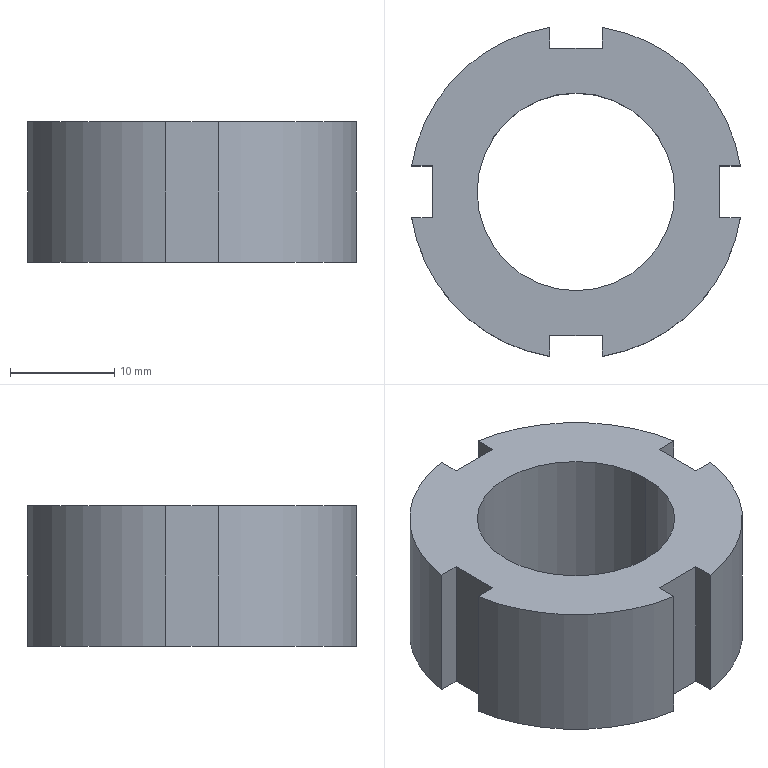Part | NX | 1 solid | 20 faces | box 31.607 x 31.607 x 13.5 mm | volume 6454 mm3 | plane 14 | cylinder 6 | commonest cylinder face diameters 32 x4 19 x2
STEP:
#1=CARTESIAN_POINT('',(-2.5,-13.803,0.));
#2=VERTEX_POINT('',#1);
#3=CARTESIAN_POINT('',(-2.5,-15.803,0.));
#4=VERTEX_POINT('',#3);
#5=CARTESIAN_POINT('',(-2.5,-13.803,0.));
#6=DIRECTION('',(0.,-1.,0.));
#7=VECTOR('',#6,1000.);
#8=LINE('',#5,#7);
#9=EDGE_CURVE('',#2,#4,#8,.T.);
#10=ORIENTED_EDGE('',*,*,#9,.T.);
#11=CARTESIAN_POINT('',(-15.803,-2.5,0.));
#12=VERTEX_POINT('',#11);
#13=CARTESIAN_POINT('',(0.,0.,0.));
#14=DIRECTION('',(0.,0.,1.));
#15=DIRECTION('',(-0.9877,-0.1563,0.));
#16=AXIS2_PLACEMENT_3D('',#13,#14,#15);
#17=CIRCLE('',#16,16.);
#18=EDGE_CURVE('',#12,#4,#17,.T.);
#19=ORIENTED_EDGE('',*,*,#18,.F.);
#20=CARTESIAN_POINT('',(-13.803,-2.5,0.));
#21=VERTEX_POINT('',#20);
#22=CARTESIAN_POINT('',(-15.803,-2.5,0.));
#23=DIRECTION('',(1.,0.,0.));
#24=VECTOR('',#23,1000.);
#25=LINE('',#22,#24);
#26=EDGE_CURVE('',#12,#21,#25,.T.);
#27=ORIENTED_EDGE('',*,*,#26,.T.);
#28=CARTESIAN_POINT('',(-13.803,2.5,0.));
#29=VERTEX_POINT('',#28);
#30=CARTESIAN_POINT('',(-13.803,-2.5,0.));
#31=DIRECTION('',(0.,1.,0.));
#32=VECTOR('',#31,1000.);
#33=LINE('',#30,#32);
#34=EDGE_CURVE('',#21,#29,#33,.T.);
#35=ORIENTED_EDGE('',*,*,#34,.T.);
#36=CARTESIAN_POINT('',(-15.803,2.5,0.));
#37=VERTEX_POINT('',#36);
#38=CARTESIAN_POINT('',(-13.803,2.5,0.));
#39=DIRECTION('',(-1.,0.,0.));
#40=VECTOR('',#39,1000.);
#41=LINE('',#38,#40);
#42=EDGE_CURVE('',#29,#37,#41,.T.);
#43=ORIENTED_EDGE('',*,*,#42,.T.);
#44=CARTESIAN_POINT('',(-2.5,15.803,0.));
#45=VERTEX_POINT('',#44);
#46=CARTESIAN_POINT('',(0.,0.,0.));
#47=DIRECTION('',(0.,0.,1.));
#48=DIRECTION('',(-0.1563,0.9877,0.));
#49=AXIS2_PLACEMENT_3D('',#46,#47,#48);
#50=CIRCLE('',#49,16.);
#51=EDGE_CURVE('',#45,#37,#50,.T.);
#52=ORIENTED_EDGE('',*,*,#51,.F.);
#53=CARTESIAN_POINT('',(-2.5,13.803,0.));
#54=VERTEX_POINT('',#53);
#55=CARTESIAN_POINT('',(-2.5,13.803,0.));
#56=DIRECTION('',(0.,1.,0.));
#57=VECTOR('',#56,1000.);
#58=LINE('',#55,#57);
#59=EDGE_CURVE('',#54,#45,#58,.T.);
#60=ORIENTED_EDGE('',*,*,#59,.F.);
#61=CARTESIAN_POINT('',(2.5,13.803,0.));
#62=VERTEX_POINT('',#61);
#63=CARTESIAN_POINT('',(2.5,13.803,0.));
#64=DIRECTION('',(-1.,0.,0.));
#65=VECTOR('',#64,1000.);
#66=LINE('',#63,#65);
#67=EDGE_CURVE('',#62,#54,#66,.T.);
#68=ORIENTED_EDGE('',*,*,#67,.F.);
#69=CARTESIAN_POINT('',(2.5,15.803,0.));
#70=VERTEX_POINT('',#69);
#71=CARTESIAN_POINT('',(2.5,15.803,0.));
#72=DIRECTION('',(0.,-1.,0.));
#73=VECTOR('',#72,1000.);
#74=LINE('',#71,#73);
#75=EDGE_CURVE('',#70,#62,#74,.T.);
#76=ORIENTED_EDGE('',*,*,#75,.F.);
#77=CARTESIAN_POINT('',(15.803,2.5,0.));
#78=VERTEX_POINT('',#77);
#79=CARTESIAN_POINT('',(0.,0.,0.));
#80=DIRECTION('',(0.,0.,1.));
#81=DIRECTION('',(0.9877,0.1563,0.));
#82=AXIS2_PLACEMENT_3D('',#79,#80,#81);
#83=CIRCLE('',#82,16.);
#84=EDGE_CURVE('',#78,#70,#83,.T.);
#85=ORIENTED_EDGE('',*,*,#84,.F.);
#86=CARTESIAN_POINT('',(13.803,2.5,0.));
#87=VERTEX_POINT('',#86);
#88=CARTESIAN_POINT('',(13.803,2.5,0.));
#89=DIRECTION('',(1.,0.,0.));
#90=VECTOR('',#89,1000.);
#91=LINE('',#88,#90);
#92=EDGE_CURVE('',#87,#78,#91,.T.);
#93=ORIENTED_EDGE('',*,*,#92,.F.);
#94=CARTESIAN_POINT('',(13.803,-2.5,0.));
#95=VERTEX_POINT('',#94);
#96=CARTESIAN_POINT('',(13.803,-2.5,0.));
#97=DIRECTION('',(0.,1.,0.));
#98=VECTOR('',#97,1000.);
#99=LINE('',#96,#98);
#100=EDGE_CURVE('',#95,#87,#99,.T.);
#101=ORIENTED_EDGE('',*,*,#100,.F.);
#102=CARTESIAN_POINT('',(15.803,-2.5,0.));
#103=VERTEX_POINT('',#102);
#104=CARTESIAN_POINT('',(15.803,-2.5,0.));
#105=DIRECTION('',(-1.,0.,0.));
#106=VECTOR('',#105,1000.);
#107=LINE('',#104,#106);
#108=EDGE_CURVE('',#103,#95,#107,.T.);
#109=ORIENTED_EDGE('',*,*,#108,.F.);
#110=CARTESIAN_POINT('',(2.5,-15.803,0.));
#111=VERTEX_POINT('',#110);
#112=CARTESIAN_POINT('',(0.,0.,0.));
#113=DIRECTION('',(0.,0.,1.));
#114=DIRECTION('',(0.1563,-0.9877,0.));
#115=AXIS2_PLACEMENT_3D('',#112,#113,#114);
#116=CIRCLE('',#115,16.);
#117=EDGE_CURVE('',#111,#103,#116,.T.);
#118=ORIENTED_EDGE('',*,*,#117,.F.);
#119=CARTESIAN_POINT('',(2.5,-13.803,0.));
#120=VERTEX_POINT('',#119);
#121=CARTESIAN_POINT('',(2.5,-15.803,0.));
#122=DIRECTION('',(0.,1.,0.));
#123=VECTOR('',#122,1000.);
#124=LINE('',#121,#123);
#125=EDGE_CURVE('',#111,#120,#124,.T.);
#126=ORIENTED_EDGE('',*,*,#125,.T.);
#127=CARTESIAN_POINT('',(2.5,-13.803,0.));
#128=DIRECTION('',(-1.,0.,0.));
#129=VECTOR('',#128,1000.);
#130=LINE('',#127,#129);
#131=EDGE_CURVE('',#120,#2,#130,.T.);
#132=ORIENTED_EDGE('',*,*,#131,.T.);
#133=EDGE_LOOP('',(#10,#19,#27,#35,#43,#52,#60,#68,#76,#85,#93,#101,#109,#118,#126,#132));
#134=FACE_BOUND('',#133,.T.);
#135=CARTESIAN_POINT('',(-9.5,0.,0.));
#136=VERTEX_POINT('',#135);
#137=CARTESIAN_POINT('',(9.5,0.,0.));
#138=VERTEX_POINT('',#137);
#139=CARTESIAN_POINT('',(0.,0.,0.));
#140=DIRECTION('',(0.,0.,-1.));
#141=DIRECTION('',(-1.,0.,0.));
#142=AXIS2_PLACEMENT_3D('',#139,#140,#141);
#143=CIRCLE('',#142,9.5);
#144=EDGE_CURVE('',#136,#138,#143,.T.);
#145=ORIENTED_EDGE('',*,*,#144,.F.);
#146=CARTESIAN_POINT('',(0.,0.,0.));
#147=DIRECTION('',(0.,0.,-1.));
#148=DIRECTION('',(-1.,0.,0.));
#149=AXIS2_PLACEMENT_3D('',#146,#147,#148);
#150=CIRCLE('',#149,9.5);
#151=EDGE_CURVE('',#138,#136,#150,.T.);
#152=ORIENTED_EDGE('',*,*,#151,.F.);
#153=EDGE_LOOP('',(#145,#152));
#154=FACE_BOUND('',#153,.T.);
#155=CARTESIAN_POINT('',(0.,0.,0.));
#156=DIRECTION('',(0.,0.,1.));
#157=DIRECTION('',(1.,0.,0.));
#158=AXIS2_PLACEMENT_3D('',#155,#156,#157);
#159=PLANE('',#158);
#160=ADVANCED_FACE('',(#134,#154),#159,.F.);
#161=ORIENTED_EDGE('',*,*,#9,.F.);
#162=CARTESIAN_POINT('',(-2.5,-13.803,13.5));
#163=VERTEX_POINT('',#162);
#164=CARTESIAN_POINT('',(-2.5,-13.803,0.));
#165=DIRECTION('',(0.,0.,1.));
#166=VECTOR('',#165,1000.);
#167=LINE('',#164,#166);
#168=EDGE_CURVE('',#2,#163,#167,.T.);
#169=ORIENTED_EDGE('',*,*,#168,.T.);
#170=CARTESIAN_POINT('',(-2.5,-15.803,13.5));
#171=VERTEX_POINT('',#170);
#172=CARTESIAN_POINT('',(-2.5,-13.803,13.5));
#173=DIRECTION('',(0.,-1.,0.));
#174=VECTOR('',#173,1000.);
#175=LINE('',#172,#174);
#176=EDGE_CURVE('',#163,#171,#175,.T.);
#177=ORIENTED_EDGE('',*,*,#176,.T.);
#178=CARTESIAN_POINT('',(-2.5,-15.803,13.5));
#179=DIRECTION('',(0.,0.,-1.));
#180=VECTOR('',#179,1000.);
#181=LINE('',#178,#180);
#182=EDGE_CURVE('',#171,#4,#181,.T.);
#183=ORIENTED_EDGE('',*,*,#182,.T.);
#184=EDGE_LOOP('',(#161,#169,#177,#183));
#185=FACE_BOUND('',#184,.T.);
#186=CARTESIAN_POINT('',(-2.5,-15.803,13.5));
#187=DIRECTION('',(1.,0.,0.));
#188=DIRECTION('',(0.,1.,0.));
#189=AXIS2_PLACEMENT_3D('',#186,#187,#188);
#190=PLANE('',#189);
#191=ADVANCED_FACE('',(#185),#190,.T.);
#192=ORIENTED_EDGE('',*,*,#182,.F.);
#193=CARTESIAN_POINT('',(-15.803,-2.5,13.5));
#194=VERTEX_POINT('',#193);
#195=CARTESIAN_POINT('',(0.,0.,13.5));
#196=DIRECTION('',(0.,0.,-1.));
#197=DIRECTION('',(-0.1563,-0.9877,0.));
#198=AXIS2_PLACEMENT_3D('',#195,#196,#197);
#199=CIRCLE('',#198,16.);
#200=EDGE_CURVE('',#171,#194,#199,.T.);
#201=ORIENTED_EDGE('',*,*,#200,.T.);
#202=CARTESIAN_POINT('',(-15.803,-2.5,0.));
#203=DIRECTION('',(0.,0.,1.));
#204=VECTOR('',#203,1000.);
#205=LINE('',#202,#204);
#206=EDGE_CURVE('',#12,#194,#205,.T.);
#207=ORIENTED_EDGE('',*,*,#206,.F.);
#208=ORIENTED_EDGE('',*,*,#18,.T.);
#209=EDGE_LOOP('',(#192,#201,#207,#208));
#210=FACE_BOUND('',#209,.T.);
#211=CARTESIAN_POINT('',(0.,0.,0.));
#212=DIRECTION('',(0.,0.,1.));
#213=DIRECTION('',(1.,0.,0.));
#214=AXIS2_PLACEMENT_3D('',#211,#212,#213);
#215=CYLINDRICAL_SURFACE('',#214,16.);
#216=ADVANCED_FACE('',(#210),#215,.T.);
#217=ORIENTED_EDGE('',*,*,#26,.F.);
#218=ORIENTED_EDGE('',*,*,#206,.T.);
#219=CARTESIAN_POINT('',(-13.803,-2.5,13.5));
#220=VERTEX_POINT('',#219);
#221=CARTESIAN_POINT('',(-15.803,-2.5,13.5));
#222=DIRECTION('',(1.,0.,0.));
#223=VECTOR('',#222,1000.);
#224=LINE('',#221,#223);
#225=EDGE_CURVE('',#194,#220,#224,.T.);
#226=ORIENTED_EDGE('',*,*,#225,.T.);
#227=CARTESIAN_POINT('',(-13.803,-2.5,0.));
#228=DIRECTION('',(0.,0.,1.));
#229=VECTOR('',#228,1000.);
#230=LINE('',#227,#229);
#231=EDGE_CURVE('',#21,#220,#230,.T.);
#232=ORIENTED_EDGE('',*,*,#231,.F.);
#233=EDGE_LOOP('',(#217,#218,#226,#232));
#234=FACE_BOUND('',#233,.T.);
#235=CARTESIAN_POINT('',(-13.803,-2.5,13.5));
#236=DIRECTION('',(0.,1.,0.));
#237=DIRECTION('',(1.,0.,0.));
#238=AXIS2_PLACEMENT_3D('',#235,#236,#237);
#239=PLANE('',#238);
#240=ADVANCED_FACE('',(#234),#239,.T.);
#241=ORIENTED_EDGE('',*,*,#34,.F.);
#242=ORIENTED_EDGE('',*,*,#231,.T.);
#243=CARTESIAN_POINT('',(-13.803,2.5,13.5));
#244=VERTEX_POINT('',#243);
#245=CARTESIAN_POINT('',(-13.803,-2.5,13.5));
#246=DIRECTION('',(0.,1.,0.));
#247=VECTOR('',#246,1000.);
#248=LINE('',#245,#247);
#249=EDGE_CURVE('',#220,#244,#248,.T.);
#250=ORIENTED_EDGE('',*,*,#249,.T.);
#251=CARTESIAN_POINT('',(-13.803,2.5,0.));
#252=DIRECTION('',(0.,0.,1.));
#253=VECTOR('',#252,1000.);
#254=LINE('',#251,#253);
#255=EDGE_CURVE('',#29,#244,#254,.T.);
#256=ORIENTED_EDGE('',*,*,#255,.F.);
#257=EDGE_LOOP('',(#241,#242,#250,#256));
#258=FACE_BOUND('',#257,.T.);
#259=CARTESIAN_POINT('',(-13.803,2.5,13.5));
#260=DIRECTION('',(-1.,0.,0.));
#261=DIRECTION('',(0.,0.,1.));
#262=AXIS2_PLACEMENT_3D('',#259,#260,#261);
#263=PLANE('',#262);
#264=ADVANCED_FACE('',(#258),#263,.T.);
#265=ORIENTED_EDGE('',*,*,#42,.F.);
#266=ORIENTED_EDGE('',*,*,#255,.T.);
#267=CARTESIAN_POINT('',(-15.803,2.5,13.5));
#268=VERTEX_POINT('',#267);
#269=CARTESIAN_POINT('',(-13.803,2.5,13.5));
#270=DIRECTION('',(-1.,0.,0.));
#271=VECTOR('',#270,1000.);
#272=LINE('',#269,#271);
#273=EDGE_CURVE('',#244,#268,#272,.T.);
#274=ORIENTED_EDGE('',*,*,#273,.T.);
#275=CARTESIAN_POINT('',(-15.803,2.5,13.5));
#276=DIRECTION('',(0.,0.,-1.));
#277=VECTOR('',#276,1000.);
#278=LINE('',#275,#277);
#279=EDGE_CURVE('',#268,#37,#278,.T.);
#280=ORIENTED_EDGE('',*,*,#279,.T.);
#281=EDGE_LOOP('',(#265,#266,#274,#280));
#282=FACE_BOUND('',#281,.T.);
#283=CARTESIAN_POINT('',(-15.803,2.5,13.5));
#284=DIRECTION('',(0.,-1.,0.));
#285=DIRECTION('',(0.,0.,-1.));
#286=AXIS2_PLACEMENT_3D('',#283,#284,#285);
#287=PLANE('',#286);
#288=ADVANCED_FACE('',(#282),#287,.T.);
#289=ORIENTED_EDGE('',*,*,#279,.F.);
#290=CARTESIAN_POINT('',(-2.5,15.803,13.5));
#291=VERTEX_POINT('',#290);
#292=CARTESIAN_POINT('',(0.,0.,13.5));
#293=DIRECTION('',(0.,0.,-1.));
#294=DIRECTION('',(-0.9877,0.1563,0.));
#295=AXIS2_PLACEMENT_3D('',#292,#293,#294);
#296=CIRCLE('',#295,16.);
#297=EDGE_CURVE('',#268,#291,#296,.T.);
#298=ORIENTED_EDGE('',*,*,#297,.T.);
#299=CARTESIAN_POINT('',(-2.5,15.803,0.));
#300=DIRECTION('',(0.,0.,1.));
#301=VECTOR('',#300,1000.);
#302=LINE('',#299,#301);
#303=EDGE_CURVE('',#45,#291,#302,.T.);
#304=ORIENTED_EDGE('',*,*,#303,.F.);
#305=ORIENTED_EDGE('',*,*,#51,.T.);
#306=EDGE_LOOP('',(#289,#298,#304,#305));
#307=FACE_BOUND('',#306,.T.);
#308=CARTESIAN_POINT('',(0.,0.,0.));
#309=DIRECTION('',(0.,0.,1.));
#310=DIRECTION('',(1.,0.,0.));
#311=AXIS2_PLACEMENT_3D('',#308,#309,#310);
#312=CYLINDRICAL_SURFACE('',#311,16.);
#313=ADVANCED_FACE('',(#307),#312,.T.);
#314=ORIENTED_EDGE('',*,*,#59,.T.);
#315=ORIENTED_EDGE('',*,*,#303,.T.);
#316=CARTESIAN_POINT('',(-2.5,13.803,13.5));
#317=VERTEX_POINT('',#316);
#318=CARTESIAN_POINT('',(-2.5,13.803,13.5));
#319=DIRECTION('',(0.,1.,0.));
#320=VECTOR('',#319,1000.);
#321=LINE('',#318,#320);
#322=EDGE_CURVE('',#317,#291,#321,.T.);
#323=ORIENTED_EDGE('',*,*,#322,.F.);
#324=CARTESIAN_POINT('',(-2.5,13.803,0.));
#325=DIRECTION('',(0.,0.,1.));
#326=VECTOR('',#325,1000.);
#327=LINE('',#324,#326);
#328=EDGE_CURVE('',#54,#317,#327,.T.);
#329=ORIENTED_EDGE('',*,*,#328,.F.);
#330=EDGE_LOOP('',(#314,#315,#323,#329));
#331=FACE_BOUND('',#330,.T.);
#332=CARTESIAN_POINT('',(-2.5,15.803,13.5));
#333=DIRECTION('',(-1.,0.,0.));
#334=DIRECTION('',(0.,0.,1.));
#335=AXIS2_PLACEMENT_3D('',#332,#333,#334);
#336=PLANE('',#335);
#337=ADVANCED_FACE('',(#331),#336,.F.);
#338=ORIENTED_EDGE('',*,*,#67,.T.);
#339=ORIENTED_EDGE('',*,*,#328,.T.);
#340=CARTESIAN_POINT('',(2.5,13.803,13.5));
#341=VERTEX_POINT('',#340);
#342=CARTESIAN_POINT('',(2.5,13.803,13.5));
#343=DIRECTION('',(-1.,0.,0.));
#344=VECTOR('',#343,1000.);
#345=LINE('',#342,#344);
#346=EDGE_CURVE('',#341,#317,#345,.T.);
#347=ORIENTED_EDGE('',*,*,#346,.F.);
#348=CARTESIAN_POINT('',(2.5,13.803,0.));
#349=DIRECTION('',(0.,0.,1.));
#350=VECTOR('',#349,1000.);
#351=LINE('',#348,#350);
#352=EDGE_CURVE('',#62,#341,#351,.T.);
#353=ORIENTED_EDGE('',*,*,#352,.F.);
#354=EDGE_LOOP('',(#338,#339,#347,#353));
#355=FACE_BOUND('',#354,.T.);
#356=CARTESIAN_POINT('',(-2.5,13.803,13.5));
#357=DIRECTION('',(0.,-1.,0.));
#358=DIRECTION('',(0.,0.,-1.));
#359=AXIS2_PLACEMENT_3D('',#356,#357,#358);
#360=PLANE('',#359);
#361=ADVANCED_FACE('',(#355),#360,.F.);
#362=ORIENTED_EDGE('',*,*,#75,.T.);
#363=ORIENTED_EDGE('',*,*,#352,.T.);
#364=CARTESIAN_POINT('',(2.5,15.803,13.5));
#365=VERTEX_POINT('',#364);
#366=CARTESIAN_POINT('',(2.5,15.803,13.5));
#367=DIRECTION('',(0.,-1.,0.));
#368=VECTOR('',#367,1000.);
#369=LINE('',#366,#368);
#370=EDGE_CURVE('',#365,#341,#369,.T.);
#371=ORIENTED_EDGE('',*,*,#370,.F.);
#372=CARTESIAN_POINT('',(2.5,15.803,13.5));
#373=DIRECTION('',(0.,0.,-1.));
#374=VECTOR('',#373,1000.);
#375=LINE('',#372,#374);
#376=EDGE_CURVE('',#365,#70,#375,.T.);
#377=ORIENTED_EDGE('',*,*,#376,.T.);
#378=EDGE_LOOP('',(#362,#363,#371,#377));
#379=FACE_BOUND('',#378,.T.);
#380=CARTESIAN_POINT('',(2.5,13.803,13.5));
#381=DIRECTION('',(1.,0.,0.));
#382=DIRECTION('',(0.,1.,0.));
#383=AXIS2_PLACEMENT_3D('',#380,#381,#382);
#384=PLANE('',#383);
#385=ADVANCED_FACE('',(#379),#384,.F.);
#386=ORIENTED_EDGE('',*,*,#84,.T.);
#387=ORIENTED_EDGE('',*,*,#376,.F.);
#388=CARTESIAN_POINT('',(15.803,2.5,13.5));
#389=VERTEX_POINT('',#388);
#390=CARTESIAN_POINT('',(0.,0.,13.5));
#391=DIRECTION('',(0.,0.,-1.));
#392=DIRECTION('',(0.1563,0.9877,0.));
#393=AXIS2_PLACEMENT_3D('',#390,#391,#392);
#394=CIRCLE('',#393,16.);
#395=EDGE_CURVE('',#365,#389,#394,.T.);
#396=ORIENTED_EDGE('',*,*,#395,.T.);
#397=CARTESIAN_POINT('',(15.803,2.5,0.));
#398=DIRECTION('',(0.,0.,1.));
#399=VECTOR('',#398,1000.);
#400=LINE('',#397,#399);
#401=EDGE_CURVE('',#78,#389,#400,.T.);
#402=ORIENTED_EDGE('',*,*,#401,.F.);
#403=EDGE_LOOP('',(#386,#387,#396,#402));
#404=FACE_BOUND('',#403,.T.);
#405=CARTESIAN_POINT('',(0.,0.,0.));
#406=DIRECTION('',(0.,0.,1.));
#407=DIRECTION('',(1.,0.,0.));
#408=AXIS2_PLACEMENT_3D('',#405,#406,#407);
#409=CYLINDRICAL_SURFACE('',#408,16.);
#410=ADVANCED_FACE('',(#404),#409,.T.);
#411=ORIENTED_EDGE('',*,*,#92,.T.);
#412=ORIENTED_EDGE('',*,*,#401,.T.);
#413=CARTESIAN_POINT('',(13.803,2.5,13.5));
#414=VERTEX_POINT('',#413);
#415=CARTESIAN_POINT('',(13.803,2.5,13.5));
#416=DIRECTION('',(1.,0.,0.));
#417=VECTOR('',#416,1000.);
#418=LINE('',#415,#417);
#419=EDGE_CURVE('',#414,#389,#418,.T.);
#420=ORIENTED_EDGE('',*,*,#419,.F.);
#421=CARTESIAN_POINT('',(13.803,2.5,0.));
#422=DIRECTION('',(0.,0.,1.));
#423=VECTOR('',#422,1000.);
#424=LINE('',#421,#423);
#425=EDGE_CURVE('',#87,#414,#424,.T.);
#426=ORIENTED_EDGE('',*,*,#425,.F.);
#427=EDGE_LOOP('',(#411,#412,#420,#426));
#428=FACE_BOUND('',#427,.T.);
#429=CARTESIAN_POINT('',(15.803,2.5,13.5));
#430=DIRECTION('',(0.,1.,0.));
#431=DIRECTION('',(1.,0.,0.));
#432=AXIS2_PLACEMENT_3D('',#429,#430,#431);
#433=PLANE('',#432);
#434=ADVANCED_FACE('',(#428),#433,.F.);
#435=ORIENTED_EDGE('',*,*,#100,.T.);
#436=ORIENTED_EDGE('',*,*,#425,.T.);
#437=CARTESIAN_POINT('',(13.803,-2.5,13.5));
#438=VERTEX_POINT('',#437);
#439=CARTESIAN_POINT('',(13.803,-2.5,13.5));
#440=DIRECTION('',(0.,1.,0.));
#441=VECTOR('',#440,1000.);
#442=LINE('',#439,#441);
#443=EDGE_CURVE('',#438,#414,#442,.T.);
#444=ORIENTED_EDGE('',*,*,#443,.F.);
#445=CARTESIAN_POINT('',(13.803,-2.5,0.));
#446=DIRECTION('',(0.,0.,1.));
#447=VECTOR('',#446,1000.);
#448=LINE('',#445,#447);
#449=EDGE_CURVE('',#95,#438,#448,.T.);
#450=ORIENTED_EDGE('',*,*,#449,.F.);
#451=EDGE_LOOP('',(#435,#436,#444,#450));
#452=FACE_BOUND('',#451,.T.);
#453=CARTESIAN_POINT('',(13.803,2.5,13.5));
#454=DIRECTION('',(-1.,0.,0.));
#455=DIRECTION('',(0.,0.,1.));
#456=AXIS2_PLACEMENT_3D('',#453,#454,#455);
#457=PLANE('',#456);
#458=ADVANCED_FACE('',(#452),#457,.F.);
#459=ORIENTED_EDGE('',*,*,#108,.T.);
#460=ORIENTED_EDGE('',*,*,#449,.T.);
#461=CARTESIAN_POINT('',(15.803,-2.5,13.5));
#462=VERTEX_POINT('',#461);
#463=CARTESIAN_POINT('',(15.803,-2.5,13.5));
#464=DIRECTION('',(-1.,0.,0.));
#465=VECTOR('',#464,1000.);
#466=LINE('',#463,#465);
#467=EDGE_CURVE('',#462,#438,#466,.T.);
#468=ORIENTED_EDGE('',*,*,#467,.F.);
#469=CARTESIAN_POINT('',(15.803,-2.5,13.5));
#470=DIRECTION('',(0.,0.,-1.));
#471=VECTOR('',#470,1000.);
#472=LINE('',#469,#471);
#473=EDGE_CURVE('',#462,#103,#472,.T.);
#474=ORIENTED_EDGE('',*,*,#473,.T.);
#475=EDGE_LOOP('',(#459,#460,#468,#474));
#476=FACE_BOUND('',#475,.T.);
#477=CARTESIAN_POINT('',(13.803,-2.5,13.5));
#478=DIRECTION('',(0.,-1.,0.));
#479=DIRECTION('',(0.,0.,-1.));
#480=AXIS2_PLACEMENT_3D('',#477,#478,#479);
#481=PLANE('',#480);
#482=ADVANCED_FACE('',(#476),#481,.F.);
#483=CARTESIAN_POINT('',(2.5,-15.803,13.5));
#484=VERTEX_POINT('',#483);
#485=CARTESIAN_POINT('',(2.5,-15.803,0.));
#486=DIRECTION('',(0.,0.,1.));
#487=VECTOR('',#486,1000.);
#488=LINE('',#485,#487);
#489=EDGE_CURVE('',#111,#484,#488,.T.);
#490=ORIENTED_EDGE('',*,*,#489,.F.);
#491=ORIENTED_EDGE('',*,*,#117,.T.);
#492=ORIENTED_EDGE('',*,*,#473,.F.);
#493=CARTESIAN_POINT('',(0.,0.,13.5));
#494=DIRECTION('',(0.,0.,-1.));
#495=DIRECTION('',(0.9877,-0.1563,0.));
#496=AXIS2_PLACEMENT_3D('',#493,#494,#495);
#497=CIRCLE('',#496,16.);
#498=EDGE_CURVE('',#462,#484,#497,.T.);
#499=ORIENTED_EDGE('',*,*,#498,.T.);
#500=EDGE_LOOP('',(#490,#491,#492,#499));
#501=FACE_BOUND('',#500,.T.);
#502=CARTESIAN_POINT('',(0.,0.,0.));
#503=DIRECTION('',(0.,0.,1.));
#504=DIRECTION('',(1.,0.,0.));
#505=AXIS2_PLACEMENT_3D('',#502,#503,#504);
#506=CYLINDRICAL_SURFACE('',#505,16.);
#507=ADVANCED_FACE('',(#501),#506,.T.);
#508=ORIENTED_EDGE('',*,*,#125,.F.);
#509=ORIENTED_EDGE('',*,*,#489,.T.);
#510=CARTESIAN_POINT('',(2.5,-13.803,13.5));
#511=VERTEX_POINT('',#510);
#512=CARTESIAN_POINT('',(2.5,-15.803,13.5));
#513=DIRECTION('',(0.,1.,0.));
#514=VECTOR('',#513,1000.);
#515=LINE('',#512,#514);
#516=EDGE_CURVE('',#484,#511,#515,.T.);
#517=ORIENTED_EDGE('',*,*,#516,.T.);
#518=CARTESIAN_POINT('',(2.5,-13.803,0.));
#519=DIRECTION('',(0.,0.,1.));
#520=VECTOR('',#519,1000.);
#521=LINE('',#518,#520);
#522=EDGE_CURVE('',#120,#511,#521,.T.);
#523=ORIENTED_EDGE('',*,*,#522,.F.);
#524=EDGE_LOOP('',(#508,#509,#517,#523));
#525=FACE_BOUND('',#524,.T.);
#526=CARTESIAN_POINT('',(2.5,-13.803,13.5));
#527=DIRECTION('',(-1.,0.,0.));
#528=DIRECTION('',(0.,0.,1.));
#529=AXIS2_PLACEMENT_3D('',#526,#527,#528);
#530=PLANE('',#529);
#531=ADVANCED_FACE('',(#525),#530,.T.);
#532=ORIENTED_EDGE('',*,*,#131,.F.);
#533=ORIENTED_EDGE('',*,*,#522,.T.);
#534=CARTESIAN_POINT('',(2.5,-13.803,13.5));
#535=DIRECTION('',(-1.,0.,0.));
#536=VECTOR('',#535,1000.);
#537=LINE('',#534,#536);
#538=EDGE_CURVE('',#511,#163,#537,.T.);
#539=ORIENTED_EDGE('',*,*,#538,.T.);
#540=ORIENTED_EDGE('',*,*,#168,.F.);
#541=EDGE_LOOP('',(#532,#533,#539,#540));
#542=FACE_BOUND('',#541,.T.);
#543=CARTESIAN_POINT('',(-2.5,-13.803,13.5));
#544=DIRECTION('',(0.,-1.,0.));
#545=DIRECTION('',(0.,0.,-1.));
#546=AXIS2_PLACEMENT_3D('',#543,#544,#545);
#547=PLANE('',#546);
#548=ADVANCED_FACE('',(#542),#547,.T.);
#549=ORIENTED_EDGE('',*,*,#176,.F.);
#550=ORIENTED_EDGE('',*,*,#538,.F.);
#551=ORIENTED_EDGE('',*,*,#516,.F.);
#552=ORIENTED_EDGE('',*,*,#498,.F.);
#553=ORIENTED_EDGE('',*,*,#467,.T.);
#554=ORIENTED_EDGE('',*,*,#443,.T.);
#555=ORIENTED_EDGE('',*,*,#419,.T.);
#556=ORIENTED_EDGE('',*,*,#395,.F.);
#557=ORIENTED_EDGE('',*,*,#370,.T.);
#558=ORIENTED_EDGE('',*,*,#346,.T.);
#559=ORIENTED_EDGE('',*,*,#322,.T.);
#560=ORIENTED_EDGE('',*,*,#297,.F.);
#561=ORIENTED_EDGE('',*,*,#273,.F.);
#562=ORIENTED_EDGE('',*,*,#249,.F.);
#563=ORIENTED_EDGE('',*,*,#225,.F.);
#564=ORIENTED_EDGE('',*,*,#200,.F.);
#565=EDGE_LOOP('',(#549,#550,#551,#552,#553,#554,#555,#556,#557,#558,#559,#560,#561,#562,#563,#564));
#566=FACE_BOUND('',#565,.T.);
#567=CARTESIAN_POINT('',(9.5,0.,13.5));
#568=VERTEX_POINT('',#567);
#569=CARTESIAN_POINT('',(-9.5,0.,13.5));
#570=VERTEX_POINT('',#569);
#571=CARTESIAN_POINT('',(0.,0.,13.5));
#572=DIRECTION('',(0.,0.,1.));
#573=DIRECTION('',(1.,0.,0.));
#574=AXIS2_PLACEMENT_3D('',#571,#572,#573);
#575=CIRCLE('',#574,9.5);
#576=EDGE_CURVE('',#568,#570,#575,.T.);
#577=ORIENTED_EDGE('',*,*,#576,.F.);
#578=CARTESIAN_POINT('',(0.,0.,13.5));
#579=DIRECTION('',(0.,0.,1.));
#580=DIRECTION('',(1.,0.,0.));
#581=AXIS2_PLACEMENT_3D('',#578,#579,#580);
#582=CIRCLE('',#581,9.5);
#583=EDGE_CURVE('',#570,#568,#582,.T.);
#584=ORIENTED_EDGE('',*,*,#583,.F.);
#585=EDGE_LOOP('',(#577,#584));
#586=FACE_BOUND('',#585,.T.);
#587=CARTESIAN_POINT('',(0.,0.,13.5));
#588=DIRECTION('',(0.,0.,1.));
#589=DIRECTION('',(1.,0.,0.));
#590=AXIS2_PLACEMENT_3D('',#587,#588,#589);
#591=PLANE('',#590);
#592=ADVANCED_FACE('',(#566,#586),#591,.T.);
#593=ORIENTED_EDGE('',*,*,#576,.T.);
#594=CARTESIAN_POINT('',(-9.5,0.,-2.092));
#595=DIRECTION('',(0.,0.,1.));
#596=VECTOR('',#595,1000.);
#597=LINE('',#594,#596);
#598=EDGE_CURVE('',#570,#136,#597,.F.);
#599=ORIENTED_EDGE('',*,*,#598,.T.);
#600=ORIENTED_EDGE('',*,*,#144,.T.);
#601=CARTESIAN_POINT('',(9.5,0.,-2.092));
#602=DIRECTION('',(0.,0.,1.));
#603=VECTOR('',#602,1000.);
#604=LINE('',#601,#603);
#605=EDGE_CURVE('',#568,#138,#604,.F.);
#606=ORIENTED_EDGE('',*,*,#605,.F.);
#607=EDGE_LOOP('',(#593,#599,#600,#606));
#608=FACE_BOUND('',#607,.T.);
#609=CARTESIAN_POINT('',(0.,0.,-2.092));
#610=DIRECTION('',(0.,0.,1.));
#611=DIRECTION('',(-1.,0.,0.));
#612=AXIS2_PLACEMENT_3D('',#609,#610,#611);
#613=CYLINDRICAL_SURFACE('',#612,9.5);
#614=ADVANCED_FACE('',(#608),#613,.F.);
#615=ORIENTED_EDGE('',*,*,#598,.F.);
#616=ORIENTED_EDGE('',*,*,#583,.T.);
#617=ORIENTED_EDGE('',*,*,#605,.T.);
#618=ORIENTED_EDGE('',*,*,#151,.T.);
#619=EDGE_LOOP('',(#615,#616,#617,#618));
#620=FACE_BOUND('',#619,.T.);
#621=CARTESIAN_POINT('',(0.,0.,-2.092));
#622=DIRECTION('',(0.,0.,1.));
#623=DIRECTION('',(-1.,0.,0.));
#624=AXIS2_PLACEMENT_3D('',#621,#622,#623);
#625=CYLINDRICAL_SURFACE('',#624,9.5);
#626=ADVANCED_FACE('',(#620),#625,.F.);
#627=CLOSED_SHELL('',(#160,#191,#216,#240,#264,#288,#313,#337,#361,#385,#410,#434,#458,#482,#507,#531,#548,#592,#614,#626));
#628=MANIFOLD_SOLID_BREP('',#627);
#629=(LENGTH_UNIT()NAMED_UNIT(*)SI_UNIT(.MILLI.,.METRE.));
#630=UNCERTAINTY_MEASURE_WITH_UNIT(LENGTH_MEASURE(0.00001),#629,'','');
#631=(NAMED_UNIT(*)PLANE_ANGLE_UNIT()SI_UNIT($,.RADIAN.));
#632=(NAMED_UNIT(*)SI_UNIT($,.STERADIAN.)SOLID_ANGLE_UNIT());
#633=(GEOMETRIC_REPRESENTATION_CONTEXT(3)GLOBAL_UNCERTAINTY_ASSIGNED_CONTEXT((#630))GLOBAL_UNIT_ASSIGNED_CONTEXT((#629,#631,#632))REPRESENTATION_CONTEXT('',''));
#634=ADVANCED_BREP_SHAPE_REPRESENTATION('',(#628),#633);